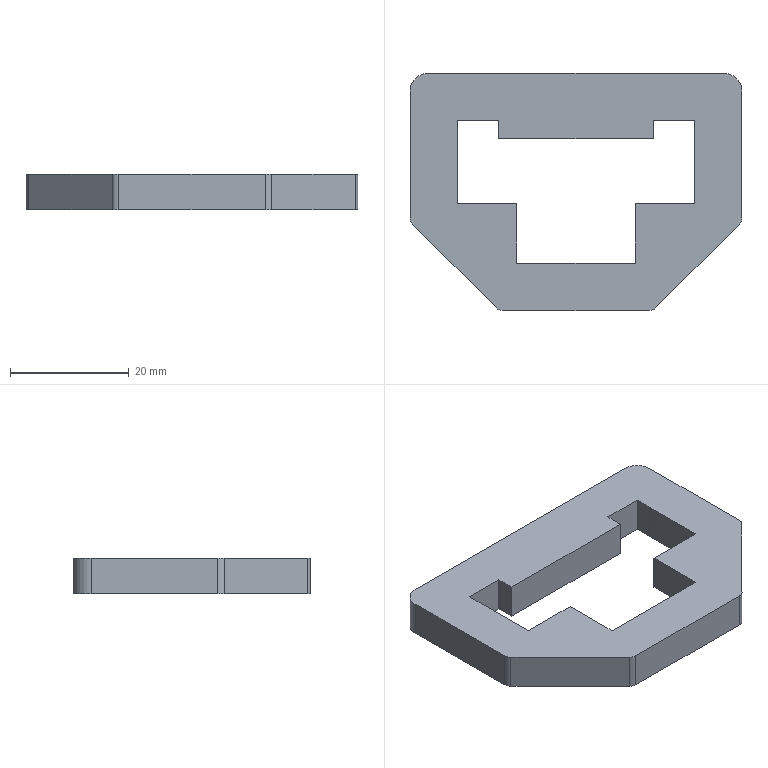Part | STEP file | JD_1_1_1_1 | 1 solid | 28 faces | box 56 x 40 x 6 mm | volume 7974 mm3 | plane 22 | cylinder 6 | commonest cylinder face diameters 3 x4 6 x2
STEP:
#1=CARTESIAN_POINT('',(0.,0.,0.));
#2=DIRECTION('',(0.,0.,1.));
#3=DIRECTION('',(1.,0.,0.));
#4=AXIS2_PLACEMENT_3D('',#1,#2,#3);
#5=CARTESIAN_POINT('',(-28.,-7.879,0.));
#6=VERTEX_POINT('',#5);
#7=CARTESIAN_POINT('',(-27.561,-8.939,0.));
#8=VERTEX_POINT('',#7);
#9=CARTESIAN_POINT('',(-26.5,-7.879,0.));
#10=DIRECTION('',(0.,0.,1.));
#11=DIRECTION('',(-1.,0.,0.));
#12=AXIS2_PLACEMENT_3D('',#9,#10,#11);
#13=CIRCLE('',#12,1.5);
#14=EDGE_CURVE('',#6,#8,#13,.T.);
#15=ORIENTED_EDGE('',*,*,#14,.T.);
#16=CARTESIAN_POINT('',(-13.439,-23.061,0.));
#17=VERTEX_POINT('',#16);
#18=CARTESIAN_POINT('',(-27.561,-8.939,0.));
#19=DIRECTION('',(0.7071,-0.7071,0.));
#20=VECTOR('',#19,19.971);
#21=LINE('',#18,#20);
#22=EDGE_CURVE('',#8,#17,#21,.T.);
#23=ORIENTED_EDGE('',*,*,#22,.T.);
#24=CARTESIAN_POINT('',(-12.379,-23.5,0.));
#25=VERTEX_POINT('',#24);
#26=CARTESIAN_POINT('',(-12.379,-22.,0.));
#27=DIRECTION('',(0.,0.,1.));
#28=DIRECTION('',(-0.7071,-0.7071,0.));
#29=AXIS2_PLACEMENT_3D('',#26,#27,#28);
#30=CIRCLE('',#29,1.5);
#31=EDGE_CURVE('',#17,#25,#30,.T.);
#32=ORIENTED_EDGE('',*,*,#31,.T.);
#33=CARTESIAN_POINT('',(12.379,-23.5,0.));
#34=VERTEX_POINT('',#33);
#35=CARTESIAN_POINT('',(12.379,-23.5,0.));
#36=DIRECTION('',(-1.,0.,0.));
#37=VECTOR('',#36,24.757);
#38=LINE('',#35,#37);
#39=EDGE_CURVE('',#34,#25,#38,.T.);
#40=ORIENTED_EDGE('',*,*,#39,.F.);
#41=CARTESIAN_POINT('',(13.439,-23.061,0.));
#42=VERTEX_POINT('',#41);
#43=CARTESIAN_POINT('',(12.379,-22.,0.));
#44=DIRECTION('',(0.,0.,1.));
#45=DIRECTION('',(0.,-1.,0.));
#46=AXIS2_PLACEMENT_3D('',#43,#44,#45);
#47=CIRCLE('',#46,1.5);
#48=EDGE_CURVE('',#34,#42,#47,.T.);
#49=ORIENTED_EDGE('',*,*,#48,.T.);
#50=CARTESIAN_POINT('',(27.561,-8.939,0.));
#51=VERTEX_POINT('',#50);
#52=CARTESIAN_POINT('',(13.439,-23.061,0.));
#53=DIRECTION('',(0.7071,0.7071,0.));
#54=VECTOR('',#53,19.971);
#55=LINE('',#52,#54);
#56=EDGE_CURVE('',#42,#51,#55,.T.);
#57=ORIENTED_EDGE('',*,*,#56,.T.);
#58=CARTESIAN_POINT('',(28.,-7.879,0.));
#59=VERTEX_POINT('',#58);
#60=CARTESIAN_POINT('',(26.5,-7.879,0.));
#61=DIRECTION('',(0.,0.,1.));
#62=DIRECTION('',(0.7071,-0.7071,0.));
#63=AXIS2_PLACEMENT_3D('',#60,#61,#62);
#64=CIRCLE('',#63,1.5);
#65=EDGE_CURVE('',#51,#59,#64,.T.);
#66=ORIENTED_EDGE('',*,*,#65,.T.);
#67=CARTESIAN_POINT('',(28.,13.5,0.));
#68=VERTEX_POINT('',#67);
#69=CARTESIAN_POINT('',(28.,13.5,0.));
#70=DIRECTION('',(0.,-1.,0.));
#71=VECTOR('',#70,21.379);
#72=LINE('',#69,#71);
#73=EDGE_CURVE('',#68,#59,#72,.T.);
#74=ORIENTED_EDGE('',*,*,#73,.F.);
#75=CARTESIAN_POINT('',(25.,16.5,0.));
#76=VERTEX_POINT('',#75);
#77=CARTESIAN_POINT('',(25.,13.5,0.));
#78=DIRECTION('',(0.,0.,1.));
#79=DIRECTION('',(1.,0.,0.));
#80=AXIS2_PLACEMENT_3D('',#77,#78,#79);
#81=CIRCLE('',#80,3.);
#82=EDGE_CURVE('',#68,#76,#81,.T.);
#83=ORIENTED_EDGE('',*,*,#82,.T.);
#84=CARTESIAN_POINT('',(-25.,16.5,0.));
#85=VERTEX_POINT('',#84);
#86=CARTESIAN_POINT('',(-25.,16.5,0.));
#87=DIRECTION('',(1.,0.,0.));
#88=VECTOR('',#87,50.);
#89=LINE('',#86,#88);
#90=EDGE_CURVE('',#85,#76,#89,.T.);
#91=ORIENTED_EDGE('',*,*,#90,.F.);
#92=CARTESIAN_POINT('',(-28.,13.5,0.));
#93=VERTEX_POINT('',#92);
#94=CARTESIAN_POINT('',(-25.,13.5,0.));
#95=DIRECTION('',(0.,0.,1.));
#96=DIRECTION('',(0.,1.,0.));
#97=AXIS2_PLACEMENT_3D('',#94,#95,#96);
#98=CIRCLE('',#97,3.);
#99=EDGE_CURVE('',#85,#93,#98,.T.);
#100=ORIENTED_EDGE('',*,*,#99,.T.);
#101=CARTESIAN_POINT('',(-28.,-7.879,0.));
#102=DIRECTION('',(0.,1.,0.));
#103=VECTOR('',#102,21.379);
#104=LINE('',#101,#103);
#105=EDGE_CURVE('',#6,#93,#104,.T.);
#106=ORIENTED_EDGE('',*,*,#105,.F.);
#107=EDGE_LOOP('',(#15,#23,#32,#40,#49,#57,#66,#74,#83,#91,#100,#106));
#108=FACE_OUTER_BOUND('',#107,.F.);
#109=CARTESIAN_POINT('',(13.,5.5,0.));
#110=VERTEX_POINT('',#109);
#111=CARTESIAN_POINT('',(13.,8.5,0.));
#112=VERTEX_POINT('',#111);
#113=CARTESIAN_POINT('',(13.,5.5,0.));
#114=DIRECTION('',(0.,1.,0.));
#115=VECTOR('',#114,3.);
#116=LINE('',#113,#115);
#117=EDGE_CURVE('',#110,#112,#116,.T.);
#118=ORIENTED_EDGE('',*,*,#117,.T.);
#119=CARTESIAN_POINT('',(20.,8.5,0.));
#120=VERTEX_POINT('',#119);
#121=CARTESIAN_POINT('',(13.,8.5,0.));
#122=DIRECTION('',(1.,0.,0.));
#123=VECTOR('',#122,7.);
#124=LINE('',#121,#123);
#125=EDGE_CURVE('',#112,#120,#124,.T.);
#126=ORIENTED_EDGE('',*,*,#125,.T.);
#127=CARTESIAN_POINT('',(20.,5.5,0.));
#128=VERTEX_POINT('',#127);
#129=CARTESIAN_POINT('',(20.,8.5,0.));
#130=DIRECTION('',(0.,-1.,0.));
#131=VECTOR('',#130,3.);
#132=LINE('',#129,#131);
#133=EDGE_CURVE('',#120,#128,#132,.T.);
#134=ORIENTED_EDGE('',*,*,#133,.T.);
#135=CARTESIAN_POINT('',(20.,-5.5,0.));
#136=VERTEX_POINT('',#135);
#137=CARTESIAN_POINT('',(20.,5.5,0.));
#138=DIRECTION('',(0.,-1.,0.));
#139=VECTOR('',#138,11.);
#140=LINE('',#137,#139);
#141=EDGE_CURVE('',#128,#136,#140,.T.);
#142=ORIENTED_EDGE('',*,*,#141,.T.);
#143=CARTESIAN_POINT('',(10.,-5.5,0.));
#144=VERTEX_POINT('',#143);
#145=CARTESIAN_POINT('',(20.,-5.5,0.));
#146=DIRECTION('',(-1.,0.,0.));
#147=VECTOR('',#146,10.);
#148=LINE('',#145,#147);
#149=EDGE_CURVE('',#136,#144,#148,.T.);
#150=ORIENTED_EDGE('',*,*,#149,.T.);
#151=CARTESIAN_POINT('',(10.,-15.5,0.));
#152=VERTEX_POINT('',#151);
#153=CARTESIAN_POINT('',(10.,-5.5,0.));
#154=DIRECTION('',(0.,-1.,0.));
#155=VECTOR('',#154,10.);
#156=LINE('',#153,#155);
#157=EDGE_CURVE('',#144,#152,#156,.T.);
#158=ORIENTED_EDGE('',*,*,#157,.T.);
#159=CARTESIAN_POINT('',(-10.,-15.5,0.));
#160=VERTEX_POINT('',#159);
#161=CARTESIAN_POINT('',(10.,-15.5,0.));
#162=DIRECTION('',(-1.,0.,0.));
#163=VECTOR('',#162,20.);
#164=LINE('',#161,#163);
#165=EDGE_CURVE('',#152,#160,#164,.T.);
#166=ORIENTED_EDGE('',*,*,#165,.T.);
#167=CARTESIAN_POINT('',(-10.,-5.5,0.));
#168=VERTEX_POINT('',#167);
#169=CARTESIAN_POINT('',(-10.,-15.5,0.));
#170=DIRECTION('',(0.,1.,0.));
#171=VECTOR('',#170,10.);
#172=LINE('',#169,#171);
#173=EDGE_CURVE('',#160,#168,#172,.T.);
#174=ORIENTED_EDGE('',*,*,#173,.T.);
#175=CARTESIAN_POINT('',(-20.,-5.5,0.));
#176=VERTEX_POINT('',#175);
#177=CARTESIAN_POINT('',(-10.,-5.5,0.));
#178=DIRECTION('',(-1.,0.,0.));
#179=VECTOR('',#178,10.);
#180=LINE('',#177,#179);
#181=EDGE_CURVE('',#168,#176,#180,.T.);
#182=ORIENTED_EDGE('',*,*,#181,.T.);
#183=CARTESIAN_POINT('',(-20.,5.5,0.));
#184=VERTEX_POINT('',#183);
#185=CARTESIAN_POINT('',(-20.,-5.5,0.));
#186=DIRECTION('',(0.,1.,0.));
#187=VECTOR('',#186,11.);
#188=LINE('',#185,#187);
#189=EDGE_CURVE('',#176,#184,#188,.T.);
#190=ORIENTED_EDGE('',*,*,#189,.T.);
#191=CARTESIAN_POINT('',(-20.,8.5,0.));
#192=VERTEX_POINT('',#191);
#193=CARTESIAN_POINT('',(-20.,5.5,0.));
#194=DIRECTION('',(0.,1.,0.));
#195=VECTOR('',#194,3.);
#196=LINE('',#193,#195);
#197=EDGE_CURVE('',#184,#192,#196,.T.);
#198=ORIENTED_EDGE('',*,*,#197,.T.);
#199=CARTESIAN_POINT('',(-13.,8.5,0.));
#200=VERTEX_POINT('',#199);
#201=CARTESIAN_POINT('',(-20.,8.5,0.));
#202=DIRECTION('',(1.,0.,0.));
#203=VECTOR('',#202,7.);
#204=LINE('',#201,#203);
#205=EDGE_CURVE('',#192,#200,#204,.T.);
#206=ORIENTED_EDGE('',*,*,#205,.T.);
#207=CARTESIAN_POINT('',(-13.,5.5,0.));
#208=VERTEX_POINT('',#207);
#209=CARTESIAN_POINT('',(-13.,8.5,0.));
#210=DIRECTION('',(0.,-1.,0.));
#211=VECTOR('',#210,3.);
#212=LINE('',#209,#211);
#213=EDGE_CURVE('',#200,#208,#212,.T.);
#214=ORIENTED_EDGE('',*,*,#213,.T.);
#215=CARTESIAN_POINT('',(-13.,5.5,0.));
#216=DIRECTION('',(1.,0.,0.));
#217=VECTOR('',#216,26.);
#218=LINE('',#215,#217);
#219=EDGE_CURVE('',#208,#110,#218,.T.);
#220=ORIENTED_EDGE('',*,*,#219,.T.);
#221=EDGE_LOOP('',(#118,#126,#134,#142,#150,#158,#166,#174,#182,#190,#198,#206,#214,#220));
#222=FACE_BOUND('',#221,.F.);
#223=CARTESIAN_POINT('',(0.,0.,0.));
#224=DIRECTION('',(0.,0.,1.));
#225=DIRECTION('',(1.,0.,0.));
#226=AXIS2_PLACEMENT_3D('',#223,#224,#225);
#227=PLANE('',#226);
#228=ADVANCED_FACE('',(#108,#222),#227,.F.);
#229=ORIENTED_EDGE('',*,*,#14,.F.);
#230=CARTESIAN_POINT('',(-28.,-7.879,6.));
#231=VERTEX_POINT('',#230);
#232=CARTESIAN_POINT('',(-28.,-7.879,0.));
#233=DIRECTION('',(0.,0.,1.));
#234=VECTOR('',#233,6.);
#235=LINE('',#232,#234);
#236=EDGE_CURVE('',#6,#231,#235,.T.);
#237=ORIENTED_EDGE('',*,*,#236,.T.);
#238=CARTESIAN_POINT('',(-27.561,-8.939,6.));
#239=VERTEX_POINT('',#238);
#240=CARTESIAN_POINT('',(-26.5,-7.879,6.));
#241=DIRECTION('',(0.,0.,-1.));
#242=DIRECTION('',(-0.7071,-0.7071,0.));
#243=AXIS2_PLACEMENT_3D('',#240,#241,#242);
#244=CIRCLE('',#243,1.5);
#245=EDGE_CURVE('',#239,#231,#244,.T.);
#246=ORIENTED_EDGE('',*,*,#245,.F.);
#247=CARTESIAN_POINT('',(-27.561,-8.939,6.));
#248=DIRECTION('',(0.,0.,-1.));
#249=VECTOR('',#248,6.);
#250=LINE('',#247,#249);
#251=EDGE_CURVE('',#239,#8,#250,.T.);
#252=ORIENTED_EDGE('',*,*,#251,.T.);
#253=EDGE_LOOP('',(#229,#237,#246,#252));
#254=FACE_OUTER_BOUND('',#253,.F.);
#255=CARTESIAN_POINT('',(-26.5,-7.879,13.822));
#256=DIRECTION('',(0.,0.,-1.));
#257=DIRECTION('',(-0.7071,-0.7071,0.));
#258=AXIS2_PLACEMENT_3D('',#255,#256,#257);
#259=CYLINDRICAL_SURFACE('',#258,1.5);
#260=ADVANCED_FACE('',(#254),#259,.T.);
#261=ORIENTED_EDGE('',*,*,#236,.F.);
#262=ORIENTED_EDGE('',*,*,#105,.T.);
#263=CARTESIAN_POINT('',(-28.,13.5,6.));
#264=VERTEX_POINT('',#263);
#265=CARTESIAN_POINT('',(-28.,13.5,6.));
#266=DIRECTION('',(0.,0.,-1.));
#267=VECTOR('',#266,6.);
#268=LINE('',#265,#267);
#269=EDGE_CURVE('',#264,#93,#268,.T.);
#270=ORIENTED_EDGE('',*,*,#269,.F.);
#271=CARTESIAN_POINT('',(-28.,13.5,6.));
#272=DIRECTION('',(0.,-1.,0.));
#273=VECTOR('',#272,21.379);
#274=LINE('',#271,#273);
#275=EDGE_CURVE('',#264,#231,#274,.T.);
#276=ORIENTED_EDGE('',*,*,#275,.T.);
#277=EDGE_LOOP('',(#261,#262,#270,#276));
#278=FACE_OUTER_BOUND('',#277,.F.);
#279=CARTESIAN_POINT('',(-28.,16.5,0.));
#280=DIRECTION('',(-1.,0.,0.));
#281=DIRECTION('',(0.,-1.,0.));
#282=AXIS2_PLACEMENT_3D('',#279,#280,#281);
#283=PLANE('',#282);
#284=ADVANCED_FACE('',(#278),#283,.T.);
#285=ORIENTED_EDGE('',*,*,#99,.F.);
#286=CARTESIAN_POINT('',(-25.,16.5,6.));
#287=VERTEX_POINT('',#286);
#288=CARTESIAN_POINT('',(-25.,16.5,0.));
#289=DIRECTION('',(0.,0.,1.));
#290=VECTOR('',#289,6.);
#291=LINE('',#288,#290);
#292=EDGE_CURVE('',#85,#287,#291,.T.);
#293=ORIENTED_EDGE('',*,*,#292,.T.);
#294=CARTESIAN_POINT('',(-25.,13.5,6.));
#295=DIRECTION('',(0.,0.,-1.));
#296=DIRECTION('',(-1.,0.,0.));
#297=AXIS2_PLACEMENT_3D('',#294,#295,#296);
#298=CIRCLE('',#297,3.);
#299=EDGE_CURVE('',#264,#287,#298,.T.);
#300=ORIENTED_EDGE('',*,*,#299,.F.);
#301=ORIENTED_EDGE('',*,*,#269,.T.);
#302=EDGE_LOOP('',(#285,#293,#300,#301));
#303=FACE_OUTER_BOUND('',#302,.F.);
#304=CARTESIAN_POINT('',(-25.,13.5,13.822));
#305=DIRECTION('',(0.,0.,-1.));
#306=DIRECTION('',(-1.,0.,0.));
#307=AXIS2_PLACEMENT_3D('',#304,#305,#306);
#308=CYLINDRICAL_SURFACE('',#307,3.);
#309=ADVANCED_FACE('',(#303),#308,.T.);
#310=ORIENTED_EDGE('',*,*,#90,.T.);
#311=CARTESIAN_POINT('',(25.,16.5,6.));
#312=VERTEX_POINT('',#311);
#313=CARTESIAN_POINT('',(25.,16.5,6.));
#314=DIRECTION('',(0.,0.,-1.));
#315=VECTOR('',#314,6.);
#316=LINE('',#313,#315);
#317=EDGE_CURVE('',#312,#76,#316,.T.);
#318=ORIENTED_EDGE('',*,*,#317,.F.);
#319=CARTESIAN_POINT('',(25.,16.5,6.));
#320=DIRECTION('',(-1.,0.,0.));
#321=VECTOR('',#320,50.);
#322=LINE('',#319,#321);
#323=EDGE_CURVE('',#312,#287,#322,.T.);
#324=ORIENTED_EDGE('',*,*,#323,.T.);
#325=ORIENTED_EDGE('',*,*,#292,.F.);
#326=EDGE_LOOP('',(#310,#318,#324,#325));
#327=FACE_OUTER_BOUND('',#326,.F.);
#328=CARTESIAN_POINT('',(-11.028,16.5,0.));
#329=DIRECTION('',(0.,1.,0.));
#330=DIRECTION('',(-1.,0.,0.));
#331=AXIS2_PLACEMENT_3D('',#328,#329,#330);
#332=PLANE('',#331);
#333=ADVANCED_FACE('',(#327),#332,.T.);
#334=ORIENTED_EDGE('',*,*,#82,.F.);
#335=CARTESIAN_POINT('',(28.,13.5,6.));
#336=VERTEX_POINT('',#335);
#337=CARTESIAN_POINT('',(28.,13.5,0.));
#338=DIRECTION('',(0.,0.,1.));
#339=VECTOR('',#338,6.);
#340=LINE('',#337,#339);
#341=EDGE_CURVE('',#68,#336,#340,.T.);
#342=ORIENTED_EDGE('',*,*,#341,.T.);
#343=CARTESIAN_POINT('',(25.,13.5,6.));
#344=DIRECTION('',(0.,0.,-1.));
#345=DIRECTION('',(0.,1.,0.));
#346=AXIS2_PLACEMENT_3D('',#343,#344,#345);
#347=CIRCLE('',#346,3.);
#348=EDGE_CURVE('',#312,#336,#347,.T.);
#349=ORIENTED_EDGE('',*,*,#348,.F.);
#350=ORIENTED_EDGE('',*,*,#317,.T.);
#351=EDGE_LOOP('',(#334,#342,#349,#350));
#352=FACE_OUTER_BOUND('',#351,.F.);
#353=CARTESIAN_POINT('',(25.,13.5,13.822));
#354=DIRECTION('',(0.,0.,-1.));
#355=DIRECTION('',(0.,1.,0.));
#356=AXIS2_PLACEMENT_3D('',#353,#354,#355);
#357=CYLINDRICAL_SURFACE('',#356,3.);
#358=ADVANCED_FACE('',(#352),#357,.T.);
#359=CARTESIAN_POINT('',(28.,-7.879,6.));
#360=VERTEX_POINT('',#359);
#361=CARTESIAN_POINT('',(28.,-7.879,6.));
#362=DIRECTION('',(0.,0.,-1.));
#363=VECTOR('',#362,6.);
#364=LINE('',#361,#363);
#365=EDGE_CURVE('',#360,#59,#364,.T.);
#366=ORIENTED_EDGE('',*,*,#365,.F.);
#367=CARTESIAN_POINT('',(28.,-7.879,6.));
#368=DIRECTION('',(0.,1.,0.));
#369=VECTOR('',#368,21.379);
#370=LINE('',#367,#369);
#371=EDGE_CURVE('',#360,#336,#370,.T.);
#372=ORIENTED_EDGE('',*,*,#371,.T.);
#373=ORIENTED_EDGE('',*,*,#341,.F.);
#374=ORIENTED_EDGE('',*,*,#73,.T.);
#375=EDGE_LOOP('',(#366,#372,#373,#374));
#376=FACE_OUTER_BOUND('',#375,.F.);
#377=CARTESIAN_POINT('',(28.,-8.5,0.));
#378=DIRECTION('',(1.,0.,0.));
#379=DIRECTION('',(0.,1.,0.));
#380=AXIS2_PLACEMENT_3D('',#377,#378,#379);
#381=PLANE('',#380);
#382=ADVANCED_FACE('',(#376),#381,.T.);
#383=ORIENTED_EDGE('',*,*,#65,.F.);
#384=CARTESIAN_POINT('',(27.561,-8.939,6.));
#385=VERTEX_POINT('',#384);
#386=CARTESIAN_POINT('',(27.561,-8.939,0.));
#387=DIRECTION('',(0.,0.,1.));
#388=VECTOR('',#387,6.);
#389=LINE('',#386,#388);
#390=EDGE_CURVE('',#51,#385,#389,.T.);
#391=ORIENTED_EDGE('',*,*,#390,.T.);
#392=CARTESIAN_POINT('',(26.5,-7.879,6.));
#393=DIRECTION('',(0.,0.,-1.));
#394=DIRECTION('',(1.,0.,0.));
#395=AXIS2_PLACEMENT_3D('',#392,#393,#394);
#396=CIRCLE('',#395,1.5);
#397=EDGE_CURVE('',#360,#385,#396,.T.);
#398=ORIENTED_EDGE('',*,*,#397,.F.);
#399=ORIENTED_EDGE('',*,*,#365,.T.);
#400=EDGE_LOOP('',(#383,#391,#398,#399));
#401=FACE_OUTER_BOUND('',#400,.F.);
#402=CARTESIAN_POINT('',(26.5,-7.879,13.822));
#403=DIRECTION('',(0.,0.,-1.));
#404=DIRECTION('',(1.,0.,0.));
#405=AXIS2_PLACEMENT_3D('',#402,#403,#404);
#406=CYLINDRICAL_SURFACE('',#405,1.5);
#407=ADVANCED_FACE('',(#401),#406,.T.);
#408=CARTESIAN_POINT('',(13.439,-23.061,6.));
#409=VERTEX_POINT('',#408);
#410=CARTESIAN_POINT('',(13.439,-23.061,6.));
#411=DIRECTION('',(0.,0.,-1.));
#412=VECTOR('',#411,6.);
#413=LINE('',#410,#412);
#414=EDGE_CURVE('',#409,#42,#413,.T.);
#415=ORIENTED_EDGE('',*,*,#414,.F.);
#416=CARTESIAN_POINT('',(27.561,-8.939,6.));
#417=DIRECTION('',(-0.7071,-0.7071,0.));
#418=VECTOR('',#417,19.971);
#419=LINE('',#416,#418);
#420=EDGE_CURVE('',#385,#409,#419,.T.);
#421=ORIENTED_EDGE('',*,*,#420,.F.);
#422=ORIENTED_EDGE('',*,*,#390,.F.);
#423=ORIENTED_EDGE('',*,*,#56,.F.);
#424=EDGE_LOOP('',(#415,#421,#422,#423));
#425=FACE_OUTER_BOUND('',#424,.F.);
#426=CARTESIAN_POINT('',(13.,-23.5,0.));
#427=DIRECTION('',(0.7071,-0.7071,0.));
#428=DIRECTION('',(0.7071,0.7071,0.));
#429=AXIS2_PLACEMENT_3D('',#426,#427,#428);
#430=PLANE('',#429);
#431=ADVANCED_FACE('',(#425),#430,.T.);
#432=ORIENTED_EDGE('',*,*,#48,.F.);
#433=CARTESIAN_POINT('',(12.379,-23.5,6.));
#434=VERTEX_POINT('',#433);
#435=CARTESIAN_POINT('',(12.379,-23.5,0.));
#436=DIRECTION('',(0.,0.,1.));
#437=VECTOR('',#436,6.);
#438=LINE('',#435,#437);
#439=EDGE_CURVE('',#34,#434,#438,.T.);
#440=ORIENTED_EDGE('',*,*,#439,.T.);
#441=CARTESIAN_POINT('',(12.379,-22.,6.));
#442=DIRECTION('',(0.,0.,-1.));
#443=DIRECTION('',(0.7071,-0.7071,0.));
#444=AXIS2_PLACEMENT_3D('',#441,#442,#443);
#445=CIRCLE('',#444,1.5);
#446=EDGE_CURVE('',#409,#434,#445,.T.);
#447=ORIENTED_EDGE('',*,*,#446,.F.);
#448=ORIENTED_EDGE('',*,*,#414,.T.);
#449=EDGE_LOOP('',(#432,#440,#447,#448));
#450=FACE_OUTER_BOUND('',#449,.F.);
#451=CARTESIAN_POINT('',(12.379,-22.,13.822));
#452=DIRECTION('',(0.,0.,-1.));
#453=DIRECTION('',(0.7071,-0.7071,0.));
#454=AXIS2_PLACEMENT_3D('',#451,#452,#453);
#455=CYLINDRICAL_SURFACE('',#454,1.5);
#456=ADVANCED_FACE('',(#450),#455,.T.);
#457=CARTESIAN_POINT('',(-12.379,-23.5,6.));
#458=VERTEX_POINT('',#457);
#459=CARTESIAN_POINT('',(-12.379,-23.5,6.));
#460=DIRECTION('',(1.,0.,0.));
#461=VECTOR('',#460,24.757);
#462=LINE('',#459,#461);
#463=EDGE_CURVE('',#458,#434,#462,.T.);
#464=ORIENTED_EDGE('',*,*,#463,.T.);
#465=ORIENTED_EDGE('',*,*,#439,.F.);
#466=ORIENTED_EDGE('',*,*,#39,.T.);
#467=CARTESIAN_POINT('',(-12.379,-23.5,6.));
#468=DIRECTION('',(0.,0.,-1.));
#469=VECTOR('',#468,6.);
#470=LINE('',#467,#469);
#471=EDGE_CURVE('',#458,#25,#470,.T.);
#472=ORIENTED_EDGE('',*,*,#471,.F.);
#473=EDGE_LOOP('',(#464,#465,#466,#472));
#474=FACE_OUTER_BOUND('',#473,.F.);
#475=CARTESIAN_POINT('',(-13.,-23.5,0.));
#476=DIRECTION('',(0.,-1.,0.));
#477=DIRECTION('',(1.,0.,0.));
#478=AXIS2_PLACEMENT_3D('',#475,#476,#477);
#479=PLANE('',#478);
#480=ADVANCED_FACE('',(#474),#479,.T.);
#481=ORIENTED_EDGE('',*,*,#245,.T.);
#482=ORIENTED_EDGE('',*,*,#275,.F.);
#483=ORIENTED_EDGE('',*,*,#299,.T.);
#484=ORIENTED_EDGE('',*,*,#323,.F.);
#485=ORIENTED_EDGE('',*,*,#348,.T.);
#486=ORIENTED_EDGE('',*,*,#371,.F.);
#487=ORIENTED_EDGE('',*,*,#397,.T.);
#488=ORIENTED_EDGE('',*,*,#420,.T.);
#489=ORIENTED_EDGE('',*,*,#446,.T.);
#490=ORIENTED_EDGE('',*,*,#463,.F.);
#491=CARTESIAN_POINT('',(-13.439,-23.061,6.));
#492=VERTEX_POINT('',#491);
#493=CARTESIAN_POINT('',(-12.379,-22.,6.));
#494=DIRECTION('',(0.,0.,-1.));
#495=DIRECTION('',(0.,-1.,0.));
#496=AXIS2_PLACEMENT_3D('',#493,#494,#495);
#497=CIRCLE('',#496,1.5);
#498=EDGE_CURVE('',#458,#492,#497,.T.);
#499=ORIENTED_EDGE('',*,*,#498,.T.);
#500=CARTESIAN_POINT('',(-13.439,-23.061,6.));
#501=DIRECTION('',(-0.7071,0.7071,0.));
#502=VECTOR('',#501,19.971);
#503=LINE('',#500,#502);
#504=EDGE_CURVE('',#492,#239,#503,.T.);
#505=ORIENTED_EDGE('',*,*,#504,.T.);
#506=EDGE_LOOP('',(#481,#482,#483,#484,#485,#486,#487,#488,#489,#490,#499,#505));
#507=FACE_OUTER_BOUND('',#506,.F.);
#508=CARTESIAN_POINT('',(13.,5.5,6.));
#509=VERTEX_POINT('',#508);
#510=CARTESIAN_POINT('',(13.,8.5,6.));
#511=VERTEX_POINT('',#510);
#512=CARTESIAN_POINT('',(13.,5.5,6.));
#513=DIRECTION('',(0.,1.,0.));
#514=VECTOR('',#513,3.);
#515=LINE('',#512,#514);
#516=EDGE_CURVE('',#509,#511,#515,.T.);
#517=ORIENTED_EDGE('',*,*,#516,.F.);
#518=CARTESIAN_POINT('',(-13.,5.5,6.));
#519=VERTEX_POINT('',#518);
#520=CARTESIAN_POINT('',(-13.,5.5,6.));
#521=DIRECTION('',(1.,0.,0.));
#522=VECTOR('',#521,26.);
#523=LINE('',#520,#522);
#524=EDGE_CURVE('',#519,#509,#523,.T.);
#525=ORIENTED_EDGE('',*,*,#524,.F.);
#526=CARTESIAN_POINT('',(-13.,8.5,6.));
#527=VERTEX_POINT('',#526);
#528=CARTESIAN_POINT('',(-13.,8.5,6.));
#529=DIRECTION('',(0.,-1.,0.));
#530=VECTOR('',#529,3.);
#531=LINE('',#528,#530);
#532=EDGE_CURVE('',#527,#519,#531,.T.);
#533=ORIENTED_EDGE('',*,*,#532,.F.);
#534=CARTESIAN_POINT('',(-20.,8.5,6.));
#535=VERTEX_POINT('',#534);
#536=CARTESIAN_POINT('',(-20.,8.5,6.));
#537=DIRECTION('',(1.,0.,0.));
#538=VECTOR('',#537,7.);
#539=LINE('',#536,#538);
#540=EDGE_CURVE('',#535,#527,#539,.T.);
#541=ORIENTED_EDGE('',*,*,#540,.F.);
#542=CARTESIAN_POINT('',(-20.,5.5,6.));
#543=VERTEX_POINT('',#542);
#544=CARTESIAN_POINT('',(-20.,5.5,6.));
#545=DIRECTION('',(0.,1.,0.));
#546=VECTOR('',#545,3.);
#547=LINE('',#544,#546);
#548=EDGE_CURVE('',#543,#535,#547,.T.);
#549=ORIENTED_EDGE('',*,*,#548,.F.);
#550=CARTESIAN_POINT('',(-20.,-5.5,6.));
#551=VERTEX_POINT('',#550);
#552=CARTESIAN_POINT('',(-20.,-5.5,6.));
#553=DIRECTION('',(0.,1.,0.));
#554=VECTOR('',#553,11.);
#555=LINE('',#552,#554);
#556=EDGE_CURVE('',#551,#543,#555,.T.);
#557=ORIENTED_EDGE('',*,*,#556,.F.);
#558=CARTESIAN_POINT('',(-10.,-5.5,6.));
#559=VERTEX_POINT('',#558);
#560=CARTESIAN_POINT('',(-10.,-5.5,6.));
#561=DIRECTION('',(-1.,0.,0.));
#562=VECTOR('',#561,10.);
#563=LINE('',#560,#562);
#564=EDGE_CURVE('',#559,#551,#563,.T.);
#565=ORIENTED_EDGE('',*,*,#564,.F.);
#566=CARTESIAN_POINT('',(-10.,-15.5,6.));
#567=VERTEX_POINT('',#566);
#568=CARTESIAN_POINT('',(-10.,-15.5,6.));
#569=DIRECTION('',(0.,1.,0.));
#570=VECTOR('',#569,10.);
#571=LINE('',#568,#570);
#572=EDGE_CURVE('',#567,#559,#571,.T.);
#573=ORIENTED_EDGE('',*,*,#572,.F.);
#574=CARTESIAN_POINT('',(10.,-15.5,6.));
#575=VERTEX_POINT('',#574);
#576=CARTESIAN_POINT('',(10.,-15.5,6.));
#577=DIRECTION('',(-1.,0.,0.));
#578=VECTOR('',#577,20.);
#579=LINE('',#576,#578);
#580=EDGE_CURVE('',#575,#567,#579,.T.);
#581=ORIENTED_EDGE('',*,*,#580,.F.);
#582=CARTESIAN_POINT('',(10.,-5.5,6.));
#583=VERTEX_POINT('',#582);
#584=CARTESIAN_POINT('',(10.,-5.5,6.));
#585=DIRECTION('',(0.,-1.,0.));
#586=VECTOR('',#585,10.);
#587=LINE('',#584,#586);
#588=EDGE_CURVE('',#583,#575,#587,.T.);
#589=ORIENTED_EDGE('',*,*,#588,.F.);
#590=CARTESIAN_POINT('',(20.,-5.5,6.));
#591=VERTEX_POINT('',#590);
#592=CARTESIAN_POINT('',(20.,-5.5,6.));
#593=DIRECTION('',(-1.,0.,0.));
#594=VECTOR('',#593,10.);
#595=LINE('',#592,#594);
#596=EDGE_CURVE('',#591,#583,#595,.T.);
#597=ORIENTED_EDGE('',*,*,#596,.F.);
#598=CARTESIAN_POINT('',(20.,5.5,6.));
#599=VERTEX_POINT('',#598);
#600=CARTESIAN_POINT('',(20.,5.5,6.));
#601=DIRECTION('',(0.,-1.,0.));
#602=VECTOR('',#601,11.);
#603=LINE('',#600,#602);
#604=EDGE_CURVE('',#599,#591,#603,.T.);
#605=ORIENTED_EDGE('',*,*,#604,.F.);
#606=CARTESIAN_POINT('',(20.,8.5,6.));
#607=VERTEX_POINT('',#606);
#608=CARTESIAN_POINT('',(20.,8.5,6.));
#609=DIRECTION('',(0.,-1.,0.));
#610=VECTOR('',#609,3.);
#611=LINE('',#608,#610);
#612=EDGE_CURVE('',#607,#599,#611,.T.);
#613=ORIENTED_EDGE('',*,*,#612,.F.);
#614=CARTESIAN_POINT('',(13.,8.5,6.));
#615=DIRECTION('',(1.,0.,0.));
#616=VECTOR('',#615,7.);
#617=LINE('',#614,#616);
#618=EDGE_CURVE('',#511,#607,#617,.T.);
#619=ORIENTED_EDGE('',*,*,#618,.F.);
#620=EDGE_LOOP('',(#517,#525,#533,#541,#549,#557,#565,#573,#581,#589,#597,#605,#613,#619));
#621=FACE_BOUND('',#620,.F.);
#622=CARTESIAN_POINT('',(0.,0.,6.));
#623=DIRECTION('',(0.,0.,1.));
#624=DIRECTION('',(1.,0.,0.));
#625=AXIS2_PLACEMENT_3D('',#622,#623,#624);
#626=PLANE('',#625);
#627=ADVANCED_FACE('',(#507,#621),#626,.T.);
#628=ORIENTED_EDGE('',*,*,#31,.F.);
#629=CARTESIAN_POINT('',(-13.439,-23.061,0.));
#630=DIRECTION('',(0.,0.,1.));
#631=VECTOR('',#630,6.);
#632=LINE('',#629,#631);
#633=EDGE_CURVE('',#17,#492,#632,.T.);
#634=ORIENTED_EDGE('',*,*,#633,.T.);
#635=ORIENTED_EDGE('',*,*,#498,.F.);
#636=ORIENTED_EDGE('',*,*,#471,.T.);
#637=EDGE_LOOP('',(#628,#634,#635,#636));
#638=FACE_OUTER_BOUND('',#637,.F.);
#639=CARTESIAN_POINT('',(-12.379,-22.,13.822));
#640=DIRECTION('',(0.,0.,-1.));
#641=DIRECTION('',(0.,-1.,0.));
#642=AXIS2_PLACEMENT_3D('',#639,#640,#641);
#643=CYLINDRICAL_SURFACE('',#642,1.5);
#644=ADVANCED_FACE('',(#638),#643,.T.);
#645=ORIENTED_EDGE('',*,*,#251,.F.);
#646=ORIENTED_EDGE('',*,*,#504,.F.);
#647=ORIENTED_EDGE('',*,*,#633,.F.);
#648=ORIENTED_EDGE('',*,*,#22,.F.);
#649=EDGE_LOOP('',(#645,#646,#647,#648));
#650=FACE_OUTER_BOUND('',#649,.F.);
#651=CARTESIAN_POINT('',(-28.,-8.5,0.));
#652=DIRECTION('',(-0.7071,-0.7071,0.));
#653=DIRECTION('',(0.7071,-0.7071,0.));
#654=AXIS2_PLACEMENT_3D('',#651,#652,#653);
#655=PLANE('',#654);
#656=ADVANCED_FACE('',(#650),#655,.T.);
#657=ORIENTED_EDGE('',*,*,#117,.F.);
#658=CARTESIAN_POINT('',(13.,5.5,0.));
#659=DIRECTION('',(0.,0.,1.));
#660=VECTOR('',#659,6.);
#661=LINE('',#658,#660);
#662=EDGE_CURVE('',#110,#509,#661,.T.);
#663=ORIENTED_EDGE('',*,*,#662,.T.);
#664=ORIENTED_EDGE('',*,*,#516,.T.);
#665=CARTESIAN_POINT('',(13.,8.5,0.));
#666=DIRECTION('',(0.,0.,1.));
#667=VECTOR('',#666,6.);
#668=LINE('',#665,#667);
#669=EDGE_CURVE('',#112,#511,#668,.T.);
#670=ORIENTED_EDGE('',*,*,#669,.F.);
#671=EDGE_LOOP('',(#657,#663,#664,#670));
#672=FACE_OUTER_BOUND('',#671,.F.);
#673=CARTESIAN_POINT('',(13.,5.5,0.));
#674=DIRECTION('',(1.,0.,0.));
#675=DIRECTION('',(0.,1.,0.));
#676=AXIS2_PLACEMENT_3D('',#673,#674,#675);
#677=PLANE('',#676);
#678=ADVANCED_FACE('',(#672),#677,.T.);
#679=ORIENTED_EDGE('',*,*,#219,.F.);
#680=CARTESIAN_POINT('',(-13.,5.5,0.));
#681=DIRECTION('',(0.,0.,1.));
#682=VECTOR('',#681,6.);
#683=LINE('',#680,#682);
#684=EDGE_CURVE('',#208,#519,#683,.T.);
#685=ORIENTED_EDGE('',*,*,#684,.T.);
#686=ORIENTED_EDGE('',*,*,#524,.T.);
#687=ORIENTED_EDGE('',*,*,#662,.F.);
#688=EDGE_LOOP('',(#679,#685,#686,#687));
#689=FACE_OUTER_BOUND('',#688,.F.);
#690=CARTESIAN_POINT('',(-13.,5.5,0.));
#691=DIRECTION('',(0.,-1.,0.));
#692=DIRECTION('',(1.,0.,0.));
#693=AXIS2_PLACEMENT_3D('',#690,#691,#692);
#694=PLANE('',#693);
#695=ADVANCED_FACE('',(#689),#694,.T.);
#696=ORIENTED_EDGE('',*,*,#213,.F.);
#697=CARTESIAN_POINT('',(-13.,8.5,0.));
#698=DIRECTION('',(0.,0.,1.));
#699=VECTOR('',#698,6.);
#700=LINE('',#697,#699);
#701=EDGE_CURVE('',#200,#527,#700,.T.);
#702=ORIENTED_EDGE('',*,*,#701,.T.);
#703=ORIENTED_EDGE('',*,*,#532,.T.);
#704=ORIENTED_EDGE('',*,*,#684,.F.);
#705=EDGE_LOOP('',(#696,#702,#703,#704));
#706=FACE_OUTER_BOUND('',#705,.F.);
#707=CARTESIAN_POINT('',(-13.,8.5,0.));
#708=DIRECTION('',(-1.,0.,0.));
#709=DIRECTION('',(0.,-1.,0.));
#710=AXIS2_PLACEMENT_3D('',#707,#708,#709);
#711=PLANE('',#710);
#712=ADVANCED_FACE('',(#706),#711,.T.);
#713=ORIENTED_EDGE('',*,*,#205,.F.);
#714=CARTESIAN_POINT('',(-20.,8.5,0.));
#715=DIRECTION('',(0.,0.,1.));
#716=VECTOR('',#715,6.);
#717=LINE('',#714,#716);
#718=EDGE_CURVE('',#192,#535,#717,.T.);
#719=ORIENTED_EDGE('',*,*,#718,.T.);
#720=ORIENTED_EDGE('',*,*,#540,.T.);
#721=ORIENTED_EDGE('',*,*,#701,.F.);
#722=EDGE_LOOP('',(#713,#719,#720,#721));
#723=FACE_OUTER_BOUND('',#722,.F.);
#724=CARTESIAN_POINT('',(-20.,8.5,0.));
#725=DIRECTION('',(0.,-1.,0.));
#726=DIRECTION('',(1.,0.,0.));
#727=AXIS2_PLACEMENT_3D('',#724,#725,#726);
#728=PLANE('',#727);
#729=ADVANCED_FACE('',(#723),#728,.T.);
#730=ORIENTED_EDGE('',*,*,#197,.F.);
#731=CARTESIAN_POINT('',(-20.,5.5,0.));
#732=DIRECTION('',(0.,0.,1.));
#733=VECTOR('',#732,6.);
#734=LINE('',#731,#733);
#735=EDGE_CURVE('',#184,#543,#734,.T.);
#736=ORIENTED_EDGE('',*,*,#735,.T.);
#737=ORIENTED_EDGE('',*,*,#548,.T.);
#738=ORIENTED_EDGE('',*,*,#718,.F.);
#739=EDGE_LOOP('',(#730,#736,#737,#738));
#740=FACE_OUTER_BOUND('',#739,.F.);
#741=CARTESIAN_POINT('',(-20.,5.5,0.));
#742=DIRECTION('',(1.,0.,0.));
#743=DIRECTION('',(0.,1.,0.));
#744=AXIS2_PLACEMENT_3D('',#741,#742,#743);
#745=PLANE('',#744);
#746=ADVANCED_FACE('',(#740),#745,.T.);
#747=ORIENTED_EDGE('',*,*,#189,.F.);
#748=CARTESIAN_POINT('',(-20.,-5.5,0.));
#749=DIRECTION('',(0.,0.,1.));
#750=VECTOR('',#749,6.);
#751=LINE('',#748,#750);
#752=EDGE_CURVE('',#176,#551,#751,.T.);
#753=ORIENTED_EDGE('',*,*,#752,.T.);
#754=ORIENTED_EDGE('',*,*,#556,.T.);
#755=ORIENTED_EDGE('',*,*,#735,.F.);
#756=EDGE_LOOP('',(#747,#753,#754,#755));
#757=FACE_OUTER_BOUND('',#756,.F.);
#758=CARTESIAN_POINT('',(-20.,-5.5,0.));
#759=DIRECTION('',(1.,0.,0.));
#760=DIRECTION('',(0.,1.,0.));
#761=AXIS2_PLACEMENT_3D('',#758,#759,#760);
#762=PLANE('',#761);
#763=ADVANCED_FACE('',(#757),#762,.T.);
#764=ORIENTED_EDGE('',*,*,#181,.F.);
#765=CARTESIAN_POINT('',(-10.,-5.5,0.));
#766=DIRECTION('',(0.,0.,1.));
#767=VECTOR('',#766,6.);
#768=LINE('',#765,#767);
#769=EDGE_CURVE('',#168,#559,#768,.T.);
#770=ORIENTED_EDGE('',*,*,#769,.T.);
#771=ORIENTED_EDGE('',*,*,#564,.T.);
#772=ORIENTED_EDGE('',*,*,#752,.F.);
#773=EDGE_LOOP('',(#764,#770,#771,#772));
#774=FACE_OUTER_BOUND('',#773,.F.);
#775=CARTESIAN_POINT('',(-10.,-5.5,0.));
#776=DIRECTION('',(0.,1.,0.));
#777=DIRECTION('',(-1.,0.,0.));
#778=AXIS2_PLACEMENT_3D('',#775,#776,#777);
#779=PLANE('',#778);
#780=ADVANCED_FACE('',(#774),#779,.T.);
#781=ORIENTED_EDGE('',*,*,#173,.F.);
#782=CARTESIAN_POINT('',(-10.,-15.5,0.));
#783=DIRECTION('',(0.,0.,1.));
#784=VECTOR('',#783,6.);
#785=LINE('',#782,#784);
#786=EDGE_CURVE('',#160,#567,#785,.T.);
#787=ORIENTED_EDGE('',*,*,#786,.T.);
#788=ORIENTED_EDGE('',*,*,#572,.T.);
#789=ORIENTED_EDGE('',*,*,#769,.F.);
#790=EDGE_LOOP('',(#781,#787,#788,#789));
#791=FACE_OUTER_BOUND('',#790,.F.);
#792=CARTESIAN_POINT('',(-10.,-15.5,0.));
#793=DIRECTION('',(1.,0.,0.));
#794=DIRECTION('',(0.,1.,0.));
#795=AXIS2_PLACEMENT_3D('',#792,#793,#794);
#796=PLANE('',#795);
#797=ADVANCED_FACE('',(#791),#796,.T.);
#798=ORIENTED_EDGE('',*,*,#165,.F.);
#799=CARTESIAN_POINT('',(10.,-15.5,0.));
#800=DIRECTION('',(0.,0.,1.));
#801=VECTOR('',#800,6.);
#802=LINE('',#799,#801);
#803=EDGE_CURVE('',#152,#575,#802,.T.);
#804=ORIENTED_EDGE('',*,*,#803,.T.);
#805=ORIENTED_EDGE('',*,*,#580,.T.);
#806=ORIENTED_EDGE('',*,*,#786,.F.);
#807=EDGE_LOOP('',(#798,#804,#805,#806));
#808=FACE_OUTER_BOUND('',#807,.F.);
#809=CARTESIAN_POINT('',(10.,-15.5,0.));
#810=DIRECTION('',(0.,1.,0.));
#811=DIRECTION('',(-1.,0.,0.));
#812=AXIS2_PLACEMENT_3D('',#809,#810,#811);
#813=PLANE('',#812);
#814=ADVANCED_FACE('',(#808),#813,.T.);
#815=ORIENTED_EDGE('',*,*,#157,.F.);
#816=CARTESIAN_POINT('',(10.,-5.5,0.));
#817=DIRECTION('',(0.,0.,1.));
#818=VECTOR('',#817,6.);
#819=LINE('',#816,#818);
#820=EDGE_CURVE('',#144,#583,#819,.T.);
#821=ORIENTED_EDGE('',*,*,#820,.T.);
#822=ORIENTED_EDGE('',*,*,#588,.T.);
#823=ORIENTED_EDGE('',*,*,#803,.F.);
#824=EDGE_LOOP('',(#815,#821,#822,#823));
#825=FACE_OUTER_BOUND('',#824,.F.);
#826=CARTESIAN_POINT('',(10.,-5.5,0.));
#827=DIRECTION('',(-1.,0.,0.));
#828=DIRECTION('',(0.,-1.,0.));
#829=AXIS2_PLACEMENT_3D('',#826,#827,#828);
#830=PLANE('',#829);
#831=ADVANCED_FACE('',(#825),#830,.T.);
#832=ORIENTED_EDGE('',*,*,#149,.F.);
#833=CARTESIAN_POINT('',(20.,-5.5,0.));
#834=DIRECTION('',(0.,0.,1.));
#835=VECTOR('',#834,6.);
#836=LINE('',#833,#835);
#837=EDGE_CURVE('',#136,#591,#836,.T.);
#838=ORIENTED_EDGE('',*,*,#837,.T.);
#839=ORIENTED_EDGE('',*,*,#596,.T.);
#840=ORIENTED_EDGE('',*,*,#820,.F.);
#841=EDGE_LOOP('',(#832,#838,#839,#840));
#842=FACE_OUTER_BOUND('',#841,.F.);
#843=CARTESIAN_POINT('',(20.,-5.5,0.));
#844=DIRECTION('',(0.,1.,0.));
#845=DIRECTION('',(-1.,0.,0.));
#846=AXIS2_PLACEMENT_3D('',#843,#844,#845);
#847=PLANE('',#846);
#848=ADVANCED_FACE('',(#842),#847,.T.);
#849=ORIENTED_EDGE('',*,*,#141,.F.);
#850=CARTESIAN_POINT('',(20.,5.5,0.));
#851=DIRECTION('',(0.,0.,1.));
#852=VECTOR('',#851,6.);
#853=LINE('',#850,#852);
#854=EDGE_CURVE('',#128,#599,#853,.T.);
#855=ORIENTED_EDGE('',*,*,#854,.T.);
#856=ORIENTED_EDGE('',*,*,#604,.T.);
#857=ORIENTED_EDGE('',*,*,#837,.F.);
#858=EDGE_LOOP('',(#849,#855,#856,#857));
#859=FACE_OUTER_BOUND('',#858,.F.);
#860=CARTESIAN_POINT('',(20.,5.5,0.));
#861=DIRECTION('',(-1.,0.,0.));
#862=DIRECTION('',(0.,-1.,0.));
#863=AXIS2_PLACEMENT_3D('',#860,#861,#862);
#864=PLANE('',#863);
#865=ADVANCED_FACE('',(#859),#864,.T.);
#866=ORIENTED_EDGE('',*,*,#133,.F.);
#867=CARTESIAN_POINT('',(20.,8.5,0.));
#868=DIRECTION('',(0.,0.,1.));
#869=VECTOR('',#868,6.);
#870=LINE('',#867,#869);
#871=EDGE_CURVE('',#120,#607,#870,.T.);
#872=ORIENTED_EDGE('',*,*,#871,.T.);
#873=ORIENTED_EDGE('',*,*,#612,.T.);
#874=ORIENTED_EDGE('',*,*,#854,.F.);
#875=EDGE_LOOP('',(#866,#872,#873,#874));
#876=FACE_OUTER_BOUND('',#875,.F.);
#877=CARTESIAN_POINT('',(20.,8.5,0.));
#878=DIRECTION('',(-1.,0.,0.));
#879=DIRECTION('',(0.,-1.,0.));
#880=AXIS2_PLACEMENT_3D('',#877,#878,#879);
#881=PLANE('',#880);
#882=ADVANCED_FACE('',(#876),#881,.T.);
#883=ORIENTED_EDGE('',*,*,#125,.F.);
#884=ORIENTED_EDGE('',*,*,#669,.T.);
#885=ORIENTED_EDGE('',*,*,#618,.T.);
#886=ORIENTED_EDGE('',*,*,#871,.F.);
#887=EDGE_LOOP('',(#883,#884,#885,#886));
#888=FACE_OUTER_BOUND('',#887,.F.);
#889=CARTESIAN_POINT('',(13.,8.5,0.));
#890=DIRECTION('',(0.,-1.,0.));
#891=DIRECTION('',(1.,0.,0.));
#892=AXIS2_PLACEMENT_3D('',#889,#890,#891);
#893=PLANE('',#892);
#894=ADVANCED_FACE('',(#888),#893,.T.);
#895=CLOSED_SHELL('',(#228,#260,#284,#309,#333,#358,#382,#407,#431,#456,#480,#627,#644,#656,#678,#695,#712,#729,#746,#763,#780,#797,#814,#831,#848,#865,#882,#894));
#896=MANIFOLD_SOLID_BREP('',#895);
#897=(LENGTH_UNIT()NAMED_UNIT(*)SI_UNIT(.MILLI.,.METRE.));
#898=UNCERTAINTY_MEASURE_WITH_UNIT(LENGTH_MEASURE(0.006908),#897,'','');
#899=(NAMED_UNIT(*)PLANE_ANGLE_UNIT()SI_UNIT($,.RADIAN.));
#900=PLANE_ANGLE_MEASURE_WITH_UNIT(PLANE_ANGLE_MEASURE(0.01745),#899);
#901=(CONVERSION_BASED_UNIT('DEGREE',#900)NAMED_UNIT(*)PLANE_ANGLE_UNIT());
#902=(NAMED_UNIT(*)SI_UNIT($,.STERADIAN.)SOLID_ANGLE_UNIT());
#903=(GEOMETRIC_REPRESENTATION_CONTEXT(3)GLOBAL_UNCERTAINTY_ASSIGNED_CONTEXT((#898))GLOBAL_UNIT_ASSIGNED_CONTEXT((#897,#901,#902))REPRESENTATION_CONTEXT('',''));
#904=ADVANCED_BREP_SHAPE_REPRESENTATION('',(#4,#896),#903);